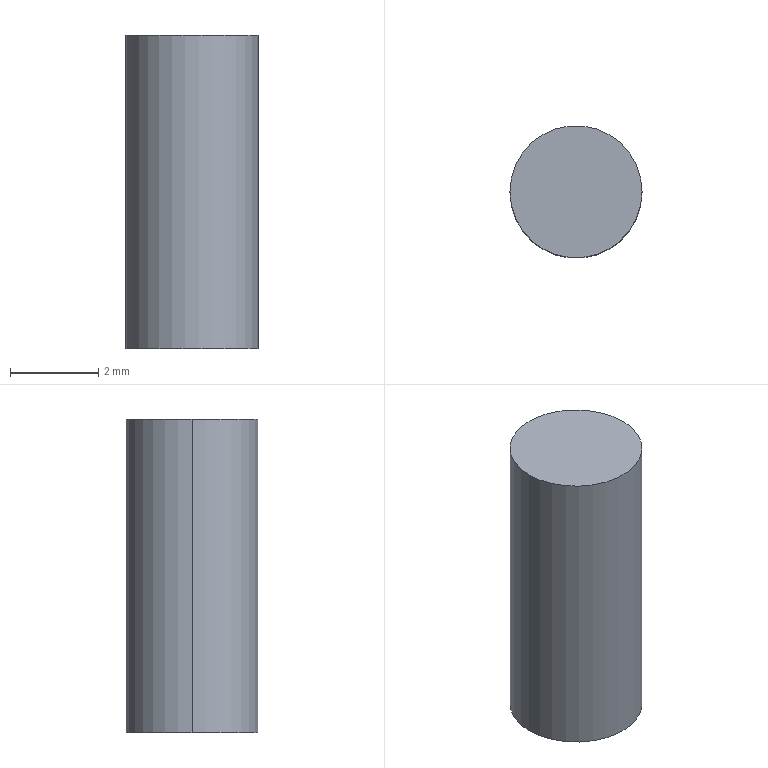Part | SolidWorks | features BaseBody 1 | 1 solid | 4 faces | box 3 x 3 x 7.119 mm | volume 50.318 mm3 | cylinder 2 | plane 2 | commonest cylinder face diameters 3 x2
STEP:
#1=CARTESIAN_POINT('',(-1.5,0.,7.119));
#2=VERTEX_POINT('',#1);
#3=CARTESIAN_POINT('',(1.5,0.,7.119));
#4=VERTEX_POINT('',#3);
#5=CARTESIAN_POINT('',(0.,0.,7.119));
#6=DIRECTION('',(0.,0.,-1.));
#7=DIRECTION('',(-1.,0.,0.));
#8=AXIS2_PLACEMENT_3D('',#5,#6,#7);
#9=CIRCLE('',#8,1.5);
#10=EDGE_CURVE('',#2,#4,#9,.T.);
#11=ORIENTED_EDGE('',*,*,#10,.T.);
#12=CARTESIAN_POINT('',(1.5,0.,0.));
#13=VERTEX_POINT('',#12);
#14=CARTESIAN_POINT('',(1.5,0.,0.));
#15=DIRECTION('',(0.,0.,-1.));
#16=VECTOR('',#15,1000.);
#17=LINE('',#14,#16);
#18=EDGE_CURVE('',#4,#13,#17,.T.);
#19=ORIENTED_EDGE('',*,*,#18,.T.);
#20=CARTESIAN_POINT('',(-1.5,0.,0.));
#21=VERTEX_POINT('',#20);
#22=CARTESIAN_POINT('',(0.,0.,0.));
#23=DIRECTION('',(0.,0.,1.));
#24=DIRECTION('',(-1.,0.,0.));
#25=AXIS2_PLACEMENT_3D('',#22,#23,#24);
#26=CIRCLE('',#25,1.5);
#27=EDGE_CURVE('',#13,#21,#26,.T.);
#28=ORIENTED_EDGE('',*,*,#27,.T.);
#29=CARTESIAN_POINT('',(-1.5,0.,0.));
#30=DIRECTION('',(0.,0.,-1.));
#31=VECTOR('',#30,1000.);
#32=LINE('',#29,#31);
#33=EDGE_CURVE('',#2,#21,#32,.T.);
#34=ORIENTED_EDGE('',*,*,#33,.F.);
#35=EDGE_LOOP('',(#11,#19,#28,#34));
#36=FACE_OUTER_BOUND('',#35,.T.);
#37=CARTESIAN_POINT('',(0.,0.,0.));
#38=DIRECTION('',(0.,0.,-1.));
#39=DIRECTION('',(-1.,0.,0.));
#40=AXIS2_PLACEMENT_3D('',#37,#38,#39);
#41=CYLINDRICAL_SURFACE('',#40,1.5);
#42=ADVANCED_FACE('',(#36),#41,.T.);
#43=ORIENTED_EDGE('',*,*,#18,.F.);
#44=CARTESIAN_POINT('',(0.,0.,7.119));
#45=DIRECTION('',(0.,0.,-1.));
#46=DIRECTION('',(-1.,0.,0.));
#47=AXIS2_PLACEMENT_3D('',#44,#45,#46);
#48=CIRCLE('',#47,1.5);
#49=EDGE_CURVE('',#4,#2,#48,.T.);
#50=ORIENTED_EDGE('',*,*,#49,.T.);
#51=ORIENTED_EDGE('',*,*,#33,.T.);
#52=CARTESIAN_POINT('',(0.,0.,0.));
#53=DIRECTION('',(0.,0.,1.));
#54=DIRECTION('',(-1.,0.,0.));
#55=AXIS2_PLACEMENT_3D('',#52,#53,#54);
#56=CIRCLE('',#55,1.5);
#57=EDGE_CURVE('',#21,#13,#56,.T.);
#58=ORIENTED_EDGE('',*,*,#57,.T.);
#59=EDGE_LOOP('',(#43,#50,#51,#58));
#60=FACE_OUTER_BOUND('',#59,.T.);
#61=CARTESIAN_POINT('',(0.,0.,0.));
#62=DIRECTION('',(0.,0.,-1.));
#63=DIRECTION('',(-1.,0.,0.));
#64=AXIS2_PLACEMENT_3D('',#61,#62,#63);
#65=CYLINDRICAL_SURFACE('',#64,1.5);
#66=ADVANCED_FACE('',(#60),#65,.T.);
#67=ORIENTED_EDGE('',*,*,#57,.F.);
#68=ORIENTED_EDGE('',*,*,#27,.F.);
#69=EDGE_LOOP('',(#67,#68));
#70=FACE_OUTER_BOUND('',#69,.T.);
#71=CARTESIAN_POINT('',(0.,0.,0.));
#72=DIRECTION('',(0.,0.,1.));
#73=DIRECTION('',(1.,0.,0.));
#74=AXIS2_PLACEMENT_3D('',#71,#72,#73);
#75=PLANE('',#74);
#76=ADVANCED_FACE('',(#70),#75,.F.);
#77=ORIENTED_EDGE('',*,*,#10,.F.);
#78=ORIENTED_EDGE('',*,*,#49,.F.);
#79=EDGE_LOOP('',(#77,#78));
#80=FACE_OUTER_BOUND('',#79,.T.);
#81=CARTESIAN_POINT('',(0.,0.,7.119));
#82=DIRECTION('',(0.,0.,1.));
#83=DIRECTION('',(1.,0.,0.));
#84=AXIS2_PLACEMENT_3D('',#81,#82,#83);
#85=PLANE('',#84);
#86=ADVANCED_FACE('',(#80),#85,.T.);
#87=CLOSED_SHELL('',(#42,#66,#76,#86));
#88=MANIFOLD_SOLID_BREP('',#87);
#89=CARTESIAN_POINT('',(0.,0.,0.));
#90=DIRECTION('',(0.,0.,1.));
#91=DIRECTION('',(1.,0.,0.));
#92=AXIS2_PLACEMENT_3D('',#89,#90,#91);
#93=(LENGTH_UNIT()NAMED_UNIT(*)SI_UNIT(.MILLI.,.METRE.));
#94=UNCERTAINTY_MEASURE_WITH_UNIT(LENGTH_MEASURE(0.00001),#93,'','');
#95=(NAMED_UNIT(*)PLANE_ANGLE_UNIT()SI_UNIT($,.RADIAN.));
#96=(NAMED_UNIT(*)SI_UNIT($,.STERADIAN.)SOLID_ANGLE_UNIT());
#97=(GEOMETRIC_REPRESENTATION_CONTEXT(3)GLOBAL_UNCERTAINTY_ASSIGNED_CONTEXT((#94))GLOBAL_UNIT_ASSIGNED_CONTEXT((#93,#95,#96))REPRESENTATION_CONTEXT('',''));
#98=ADVANCED_BREP_SHAPE_REPRESENTATION('',(#88,#92),#97);